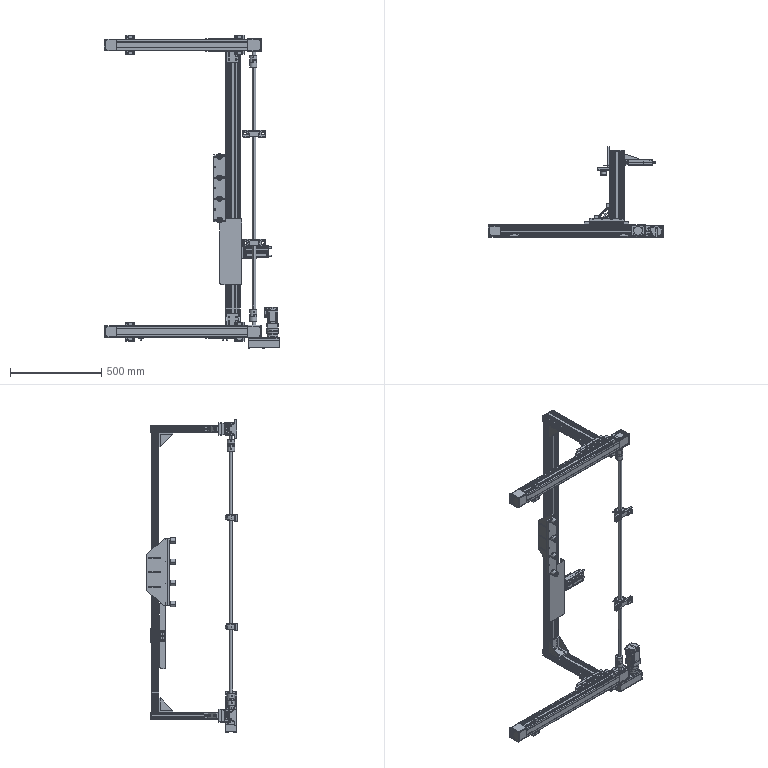Part | SolidWorks | 66 solids | 7235 faces | volume 11809484 mm3 | plane 3371 | cylinder 2266 | cone 1009 | spline 488 | torus 81 | sphere 20 | commonest cylinder face diameters 1 x170 8 x137 5.5 x136 2 x112 0.6 x106 4 x102